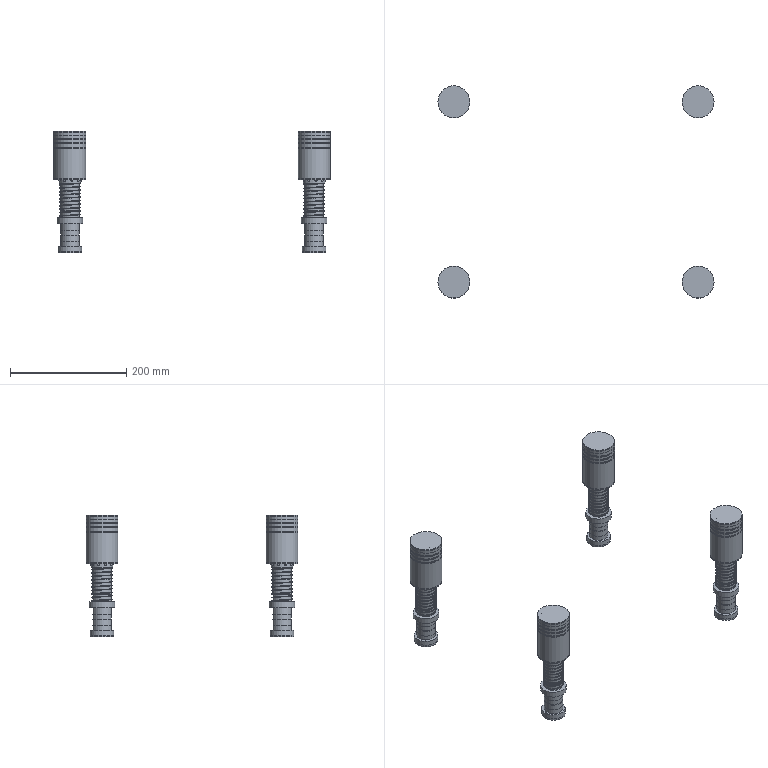Part | NX | features BREP 11 | 44 solids | 1008 faces | box 475 x 365 x 209 mm | volume 4104136 mm3 | sphere 648 | plane 172 | cylinder 144 | torus 32 | cone 8 | spline 4 | commonest cylinder face diameters 32 x20 54.996 x16 44 x12 52.246 x12 8 x8 10 x8